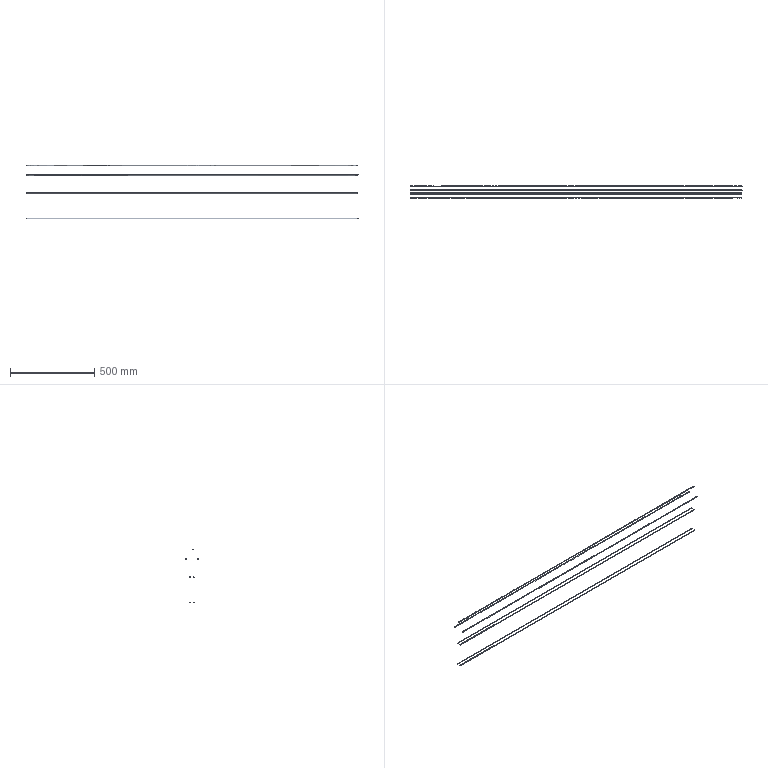Part | SolidWorks | features BaseBody 7 | 7 solids | 28 faces | box 1975 x 72.517 x 321.142 mm | volume 173509 mm3 | spline 14 | plane 14
STEP:
#1=CARTESIAN_POINT('',(28.5,0.007462,-18.003));
#2=VERTEX_POINT('',#1);
#3=CARTESIAN_POINT('',(2000.,0.5236,-17.996));
#4=VERTEX_POINT('',#3);
#5=CARTESIAN_POINT('',(1014.25,0.2655,-18.));
#6=DIRECTION('',(1.,0.0002618,0.000003427));
#7=VECTOR('',#6,1000.);
#8=LINE('',#5,#7);
#9=EDGE_CURVE('',#2,#4,#8,.T.);
#10=ORIENTED_EDGE('',*,*,#9,.F.);
#11=CARTESIAN_POINT('',(28.5,0.007462,-22.003));
#12=VERTEX_POINT('',#11);
#13=CARTESIAN_POINT('',(28.5,0.007462,-22.003));
#14=CARTESIAN_POINT('',(28.5,-3.993,-22.003));
#15=CARTESIAN_POINT('',(28.5,-3.993,-18.003));
#16=CARTESIAN_POINT('',(28.5,0.007462,-18.003));
#17=(BOUNDED_CURVE()B_SPLINE_CURVE(3,(#13,#14,#15,#16),.UNSPECIFIED.,.F.,.F.)B_SPLINE_CURVE_WITH_KNOTS((4,4),(0.,0.006252),.UNSPECIFIED.)CURVE()GEOMETRIC_REPRESENTATION_ITEM()RATIONAL_B_SPLINE_CURVE((1.,0.3333,0.3333,1.))REPRESENTATION_ITEM(''));
#18=EDGE_CURVE('',#12,#2,#17,.T.);
#19=ORIENTED_EDGE('',*,*,#18,.F.);
#20=CARTESIAN_POINT('',(2000.,0.5236,-21.996));
#21=VERTEX_POINT('',#20);
#22=CARTESIAN_POINT('',(1014.25,0.2655,-22.));
#23=DIRECTION('',(-1.,-0.0002618,-0.000003427));
#24=VECTOR('',#23,1000.);
#25=LINE('',#22,#24);
#26=EDGE_CURVE('',#21,#12,#25,.T.);
#27=ORIENTED_EDGE('',*,*,#26,.F.);
#28=CARTESIAN_POINT('',(2000.,0.5236,-17.996));
#29=CARTESIAN_POINT('',(2000.,-3.476,-17.996));
#30=CARTESIAN_POINT('',(2000.,-3.476,-21.996));
#31=CARTESIAN_POINT('',(2000.,0.5236,-21.996));
#32=(BOUNDED_CURVE()B_SPLINE_CURVE(3,(#28,#29,#30,#31),.UNSPECIFIED.,.F.,.F.)B_SPLINE_CURVE_WITH_KNOTS((4,4),(0.,0.006252),.UNSPECIFIED.)CURVE()GEOMETRIC_REPRESENTATION_ITEM()RATIONAL_B_SPLINE_CURVE((1.,0.3333,0.3333,1.))REPRESENTATION_ITEM(''));
#33=EDGE_CURVE('',#4,#21,#32,.T.);
#34=ORIENTED_EDGE('',*,*,#33,.F.);
#35=EDGE_LOOP('',(#10,#19,#27,#34));
#36=FACE_OUTER_BOUND('',#35,.T.);
#37=CARTESIAN_POINT('',(2000.,0.5236,-17.996));
#38=CARTESIAN_POINT('',(28.5,0.007462,-18.003));
#39=CARTESIAN_POINT('',(2000.,-3.476,-17.996));
#40=CARTESIAN_POINT('',(28.5,-3.993,-18.003));
#41=CARTESIAN_POINT('',(2000.,-3.476,-21.996));
#42=CARTESIAN_POINT('',(28.5,-3.993,-22.003));
#43=CARTESIAN_POINT('',(2000.,0.5236,-21.996));
#44=CARTESIAN_POINT('',(28.5,0.007462,-22.003));
#45=(BOUNDED_SURFACE()B_SPLINE_SURFACE(3,1,((#37,#38),(#39,#40),(#41,#42),(#43,#44)),.UNSPECIFIED.,.F.,.F.,.F.)B_SPLINE_SURFACE_WITH_KNOTS((4,4),(2,2),(0.,1.),(0.,1.),.UNSPECIFIED.)GEOMETRIC_REPRESENTATION_ITEM()RATIONAL_B_SPLINE_SURFACE(((1.,1.),(0.3333,0.3333),(0.3333,0.3333),(1.,1.)))REPRESENTATION_ITEM('')SURFACE());
#46=ADVANCED_FACE('',(#36),#45,.F.);
#47=CARTESIAN_POINT('',(2000.,0.5236,-21.996));
#48=CARTESIAN_POINT('',(2000.,4.524,-21.996));
#49=CARTESIAN_POINT('',(2000.,4.524,-17.996));
#50=CARTESIAN_POINT('',(2000.,0.5236,-17.996));
#51=(BOUNDED_CURVE()B_SPLINE_CURVE(3,(#47,#48,#49,#50),.UNSPECIFIED.,.F.,.F.)B_SPLINE_CURVE_WITH_KNOTS((4,4),(0.,0.006252),.UNSPECIFIED.)CURVE()GEOMETRIC_REPRESENTATION_ITEM()RATIONAL_B_SPLINE_CURVE((1.,0.3333,0.3333,1.))REPRESENTATION_ITEM(''));
#52=EDGE_CURVE('',#21,#4,#51,.T.);
#53=ORIENTED_EDGE('',*,*,#52,.T.);
#54=ORIENTED_EDGE('',*,*,#33,.T.);
#55=EDGE_LOOP('',(#53,#54));
#56=FACE_OUTER_BOUND('',#55,.T.);
#57=CARTESIAN_POINT('',(2000.,-1.5,-17.972));
#58=DIRECTION('',(1.,0.,0.));
#59=DIRECTION('',(0.,0.,-1.));
#60=AXIS2_PLACEMENT_3D('',#57,#58,#59);
#61=PLANE('',#60);
#62=ADVANCED_FACE('',(#56),#61,.T.);
#63=ORIENTED_EDGE('',*,*,#52,.F.);
#64=ORIENTED_EDGE('',*,*,#26,.T.);
#65=CARTESIAN_POINT('',(28.5,0.007462,-18.003));
#66=CARTESIAN_POINT('',(28.5,4.007,-18.003));
#67=CARTESIAN_POINT('',(28.5,4.007,-22.003));
#68=CARTESIAN_POINT('',(28.5,0.007462,-22.003));
#69=(BOUNDED_CURVE()B_SPLINE_CURVE(3,(#65,#66,#67,#68),.UNSPECIFIED.,.F.,.F.)B_SPLINE_CURVE_WITH_KNOTS((4,4),(0.,0.006252),.UNSPECIFIED.)CURVE()GEOMETRIC_REPRESENTATION_ITEM()RATIONAL_B_SPLINE_CURVE((1.,0.3333,0.3333,1.))REPRESENTATION_ITEM(''));
#70=EDGE_CURVE('',#2,#12,#69,.T.);
#71=ORIENTED_EDGE('',*,*,#70,.F.);
#72=ORIENTED_EDGE('',*,*,#9,.T.);
#73=EDGE_LOOP('',(#63,#64,#71,#72));
#74=FACE_OUTER_BOUND('',#73,.T.);
#75=CARTESIAN_POINT('',(2000.,0.5236,-21.996));
#76=CARTESIAN_POINT('',(28.5,0.007462,-22.003));
#77=CARTESIAN_POINT('',(2000.,4.524,-21.996));
#78=CARTESIAN_POINT('',(28.5,4.007,-22.003));
#79=CARTESIAN_POINT('',(2000.,4.524,-17.996));
#80=CARTESIAN_POINT('',(28.5,4.007,-18.003));
#81=CARTESIAN_POINT('',(2000.,0.5236,-17.996));
#82=CARTESIAN_POINT('',(28.5,0.007462,-18.003));
#83=(BOUNDED_SURFACE()B_SPLINE_SURFACE(3,1,((#75,#76),(#77,#78),(#79,#80),(#81,#82)),.UNSPECIFIED.,.F.,.F.,.F.)B_SPLINE_SURFACE_WITH_KNOTS((4,4),(2,2),(0.,1.),(0.,1.),.UNSPECIFIED.)GEOMETRIC_REPRESENTATION_ITEM()RATIONAL_B_SPLINE_SURFACE(((1.,1.),(0.3333,0.3333),(0.3333,0.3333),(1.,1.)))REPRESENTATION_ITEM('')SURFACE());
#84=ADVANCED_FACE('',(#74),#83,.F.);
#85=ORIENTED_EDGE('',*,*,#18,.T.);
#86=ORIENTED_EDGE('',*,*,#70,.T.);
#87=EDGE_LOOP('',(#85,#86));
#88=FACE_OUTER_BOUND('',#87,.T.);
#89=CARTESIAN_POINT('',(28.5,-2.017,-22.027));
#90=DIRECTION('',(-1.,0.,0.));
#91=DIRECTION('',(0.,0.,1.));
#92=AXIS2_PLACEMENT_3D('',#89,#90,#91);
#93=PLANE('',#92);
#94=ADVANCED_FACE('',(#88),#93,.T.);
#95=CLOSED_SHELL('',(#46,#62,#84,#94));
#96=MANIFOLD_SOLID_BREP('',#95);
#97=CARTESIAN_POINT('',(28.5,0.007462,-169.026));
#98=VERTEX_POINT('',#97);
#99=CARTESIAN_POINT('',(2000.,0.5236,-169.019));
#100=VERTEX_POINT('',#99);
#101=CARTESIAN_POINT('',(1014.25,0.2655,-169.023));
#102=DIRECTION('',(1.,0.0002618,0.000003427));
#103=VECTOR('',#102,1000.);
#104=LINE('',#101,#103);
#105=EDGE_CURVE('',#98,#100,#104,.T.);
#106=ORIENTED_EDGE('',*,*,#105,.F.);
#107=CARTESIAN_POINT('',(28.5,0.007462,-173.026));
#108=VERTEX_POINT('',#107);
#109=CARTESIAN_POINT('',(28.5,0.007462,-173.026));
#110=CARTESIAN_POINT('',(28.5,-3.993,-173.026));
#111=CARTESIAN_POINT('',(28.5,-3.993,-169.026));
#112=CARTESIAN_POINT('',(28.5,0.007462,-169.026));
#113=(BOUNDED_CURVE()B_SPLINE_CURVE(3,(#109,#110,#111,#112),.UNSPECIFIED.,.F.,.F.)B_SPLINE_CURVE_WITH_KNOTS((4,4),(0.,0.006252),.UNSPECIFIED.)CURVE()GEOMETRIC_REPRESENTATION_ITEM()RATIONAL_B_SPLINE_CURVE((1.,0.3333,0.3333,1.))REPRESENTATION_ITEM(''));
#114=EDGE_CURVE('',#108,#98,#113,.T.);
#115=ORIENTED_EDGE('',*,*,#114,.F.);
#116=CARTESIAN_POINT('',(2000.,0.5236,-173.019));
#117=VERTEX_POINT('',#116);
#118=CARTESIAN_POINT('',(1014.25,0.2655,-173.023));
#119=DIRECTION('',(-1.,-0.0002618,-0.000003427));
#120=VECTOR('',#119,1000.);
#121=LINE('',#118,#120);
#122=EDGE_CURVE('',#117,#108,#121,.T.);
#123=ORIENTED_EDGE('',*,*,#122,.F.);
#124=CARTESIAN_POINT('',(2000.,0.5236,-169.019));
#125=CARTESIAN_POINT('',(2000.,-3.476,-169.019));
#126=CARTESIAN_POINT('',(2000.,-3.476,-173.019));
#127=CARTESIAN_POINT('',(2000.,0.5236,-173.019));
#128=(BOUNDED_CURVE()B_SPLINE_CURVE(3,(#124,#125,#126,#127),.UNSPECIFIED.,.F.,.F.)B_SPLINE_CURVE_WITH_KNOTS((4,4),(0.,0.006252),.UNSPECIFIED.)CURVE()GEOMETRIC_REPRESENTATION_ITEM()RATIONAL_B_SPLINE_CURVE((1.,0.3333,0.3333,1.))REPRESENTATION_ITEM(''));
#129=EDGE_CURVE('',#100,#117,#128,.T.);
#130=ORIENTED_EDGE('',*,*,#129,.F.);
#131=EDGE_LOOP('',(#106,#115,#123,#130));
#132=FACE_OUTER_BOUND('',#131,.T.);
#133=CARTESIAN_POINT('',(2000.,0.5236,-169.019));
#134=CARTESIAN_POINT('',(28.5,0.007462,-169.026));
#135=CARTESIAN_POINT('',(2000.,-3.476,-169.019));
#136=CARTESIAN_POINT('',(28.5,-3.993,-169.026));
#137=CARTESIAN_POINT('',(2000.,-3.476,-173.019));
#138=CARTESIAN_POINT('',(28.5,-3.993,-173.026));
#139=CARTESIAN_POINT('',(2000.,0.5236,-173.019));
#140=CARTESIAN_POINT('',(28.5,0.007462,-173.026));
#141=(BOUNDED_SURFACE()B_SPLINE_SURFACE(3,1,((#133,#134),(#135,#136),(#137,#138),(#139,#140)),.UNSPECIFIED.,.F.,.F.,.T.)B_SPLINE_SURFACE_WITH_KNOTS((4,4),(2,2),(0.,1.),(0.,1.),.UNSPECIFIED.)GEOMETRIC_REPRESENTATION_ITEM()RATIONAL_B_SPLINE_SURFACE(((1.,1.),(0.3333,0.3333),(0.3333,0.3333),(1.,1.)))REPRESENTATION_ITEM('')SURFACE());
#142=ADVANCED_FACE('',(#132),#141,.F.);
#143=CARTESIAN_POINT('',(2000.,0.5236,-173.019));
#144=CARTESIAN_POINT('',(2000.,4.524,-173.019));
#145=CARTESIAN_POINT('',(2000.,4.524,-169.019));
#146=CARTESIAN_POINT('',(2000.,0.5236,-169.019));
#147=(BOUNDED_CURVE()B_SPLINE_CURVE(3,(#143,#144,#145,#146),.UNSPECIFIED.,.F.,.F.)B_SPLINE_CURVE_WITH_KNOTS((4,4),(0.,0.006252),.UNSPECIFIED.)CURVE()GEOMETRIC_REPRESENTATION_ITEM()RATIONAL_B_SPLINE_CURVE((1.,0.3333,0.3333,1.))REPRESENTATION_ITEM(''));
#148=EDGE_CURVE('',#117,#100,#147,.T.);
#149=ORIENTED_EDGE('',*,*,#148,.T.);
#150=ORIENTED_EDGE('',*,*,#129,.T.);
#151=EDGE_LOOP('',(#149,#150));
#152=FACE_OUTER_BOUND('',#151,.T.);
#153=CARTESIAN_POINT('',(2000.,-1.5,-168.995));
#154=DIRECTION('',(1.,0.,0.));
#155=DIRECTION('',(0.,0.,-1.));
#156=AXIS2_PLACEMENT_3D('',#153,#154,#155);
#157=PLANE('',#156);
#158=ADVANCED_FACE('',(#152),#157,.T.);
#159=ORIENTED_EDGE('',*,*,#148,.F.);
#160=ORIENTED_EDGE('',*,*,#122,.T.);
#161=CARTESIAN_POINT('',(28.5,0.007462,-169.026));
#162=CARTESIAN_POINT('',(28.5,4.007,-169.026));
#163=CARTESIAN_POINT('',(28.5,4.007,-173.026));
#164=CARTESIAN_POINT('',(28.5,0.007462,-173.026));
#165=(BOUNDED_CURVE()B_SPLINE_CURVE(3,(#161,#162,#163,#164),.UNSPECIFIED.,.F.,.F.)B_SPLINE_CURVE_WITH_KNOTS((4,4),(0.,0.006252),.UNSPECIFIED.)CURVE()GEOMETRIC_REPRESENTATION_ITEM()RATIONAL_B_SPLINE_CURVE((1.,0.3333,0.3333,1.))REPRESENTATION_ITEM(''));
#166=EDGE_CURVE('',#98,#108,#165,.T.);
#167=ORIENTED_EDGE('',*,*,#166,.F.);
#168=ORIENTED_EDGE('',*,*,#105,.T.);
#169=EDGE_LOOP('',(#159,#160,#167,#168));
#170=FACE_OUTER_BOUND('',#169,.T.);
#171=CARTESIAN_POINT('',(2000.,0.5236,-173.019));
#172=CARTESIAN_POINT('',(28.5,0.007462,-173.026));
#173=CARTESIAN_POINT('',(2000.,4.524,-173.019));
#174=CARTESIAN_POINT('',(28.5,4.007,-173.026));
#175=CARTESIAN_POINT('',(2000.,4.524,-169.019));
#176=CARTESIAN_POINT('',(28.5,4.007,-169.026));
#177=CARTESIAN_POINT('',(2000.,0.5236,-169.019));
#178=CARTESIAN_POINT('',(28.5,0.007462,-169.026));
#179=(BOUNDED_SURFACE()B_SPLINE_SURFACE(3,1,((#171,#172),(#173,#174),(#175,#176),(#177,#178)),.UNSPECIFIED.,.F.,.F.,.F.)B_SPLINE_SURFACE_WITH_KNOTS((4,4),(2,2),(0.,1.),(0.,1.),.UNSPECIFIED.)GEOMETRIC_REPRESENTATION_ITEM()RATIONAL_B_SPLINE_SURFACE(((1.,1.),(0.3333,0.3333),(0.3333,0.3333),(1.,1.)))REPRESENTATION_ITEM('')SURFACE());
#180=ADVANCED_FACE('',(#170),#179,.F.);
#181=ORIENTED_EDGE('',*,*,#114,.T.);
#182=ORIENTED_EDGE('',*,*,#166,.T.);
#183=EDGE_LOOP('',(#181,#182));
#184=FACE_OUTER_BOUND('',#183,.T.);
#185=CARTESIAN_POINT('',(28.5,-2.017,-173.05));
#186=DIRECTION('',(-1.,0.,0.));
#187=DIRECTION('',(0.,0.,1.));
#188=AXIS2_PLACEMENT_3D('',#185,#186,#187);
#189=PLANE('',#188);
#190=ADVANCED_FACE('',(#184),#189,.T.);
#191=CLOSED_SHELL('',(#142,#158,#180,#190));
#192=MANIFOLD_SOLID_BREP('',#191);
#193=CARTESIAN_POINT('',(28.5,22.007,-168.642));
#194=VERTEX_POINT('',#193);
#195=CARTESIAN_POINT('',(2000.,22.524,-168.635));
#196=VERTEX_POINT('',#195);
#197=CARTESIAN_POINT('',(1014.25,22.266,-168.639));
#198=DIRECTION('',(1.,0.0002618,0.000003427));
#199=VECTOR('',#198,1000.);
#200=LINE('',#197,#199);
#201=EDGE_CURVE('',#194,#196,#200,.T.);
#202=ORIENTED_EDGE('',*,*,#201,.F.);
#203=CARTESIAN_POINT('',(28.5,22.007,-172.642));
#204=VERTEX_POINT('',#203);
#205=CARTESIAN_POINT('',(28.5,22.007,-172.642));
#206=CARTESIAN_POINT('',(28.5,18.007,-172.642));
#207=CARTESIAN_POINT('',(28.5,18.007,-168.642));
#208=CARTESIAN_POINT('',(28.5,22.007,-168.642));
#209=(BOUNDED_CURVE()B_SPLINE_CURVE(3,(#205,#206,#207,#208),.UNSPECIFIED.,.F.,.F.)B_SPLINE_CURVE_WITH_KNOTS((4,4),(0.,0.006252),.UNSPECIFIED.)CURVE()GEOMETRIC_REPRESENTATION_ITEM()RATIONAL_B_SPLINE_CURVE((1.,0.3333,0.3333,1.))REPRESENTATION_ITEM(''));
#210=EDGE_CURVE('',#204,#194,#209,.T.);
#211=ORIENTED_EDGE('',*,*,#210,.F.);
#212=CARTESIAN_POINT('',(2000.,22.524,-172.635));
#213=VERTEX_POINT('',#212);
#214=CARTESIAN_POINT('',(1014.25,22.266,-172.639));
#215=DIRECTION('',(-1.,-0.0002618,-0.000003427));
#216=VECTOR('',#215,1000.);
#217=LINE('',#214,#216);
#218=EDGE_CURVE('',#213,#204,#217,.T.);
#219=ORIENTED_EDGE('',*,*,#218,.F.);
#220=CARTESIAN_POINT('',(2000.,22.524,-168.635));
#221=CARTESIAN_POINT('',(2000.,18.524,-168.635));
#222=CARTESIAN_POINT('',(2000.,18.524,-172.635));
#223=CARTESIAN_POINT('',(2000.,22.524,-172.635));
#224=(BOUNDED_CURVE()B_SPLINE_CURVE(3,(#220,#221,#222,#223),.UNSPECIFIED.,.F.,.F.)B_SPLINE_CURVE_WITH_KNOTS((4,4),(0.,0.006252),.UNSPECIFIED.)CURVE()GEOMETRIC_REPRESENTATION_ITEM()RATIONAL_B_SPLINE_CURVE((1.,0.3333,0.3333,1.))REPRESENTATION_ITEM(''));
#225=EDGE_CURVE('',#196,#213,#224,.T.);
#226=ORIENTED_EDGE('',*,*,#225,.F.);
#227=EDGE_LOOP('',(#202,#211,#219,#226));
#228=FACE_OUTER_BOUND('',#227,.T.);
#229=CARTESIAN_POINT('',(2000.,22.524,-168.635));
#230=CARTESIAN_POINT('',(28.5,22.007,-168.642));
#231=CARTESIAN_POINT('',(2000.,18.524,-168.635));
#232=CARTESIAN_POINT('',(28.5,18.007,-168.642));
#233=CARTESIAN_POINT('',(2000.,18.524,-172.635));
#234=CARTESIAN_POINT('',(28.5,18.007,-172.642));
#235=CARTESIAN_POINT('',(2000.,22.524,-172.635));
#236=CARTESIAN_POINT('',(28.5,22.007,-172.642));
#237=(BOUNDED_SURFACE()B_SPLINE_SURFACE(3,1,((#229,#230),(#231,#232),(#233,#234),(#235,#236)),.UNSPECIFIED.,.F.,.F.,.F.)B_SPLINE_SURFACE_WITH_KNOTS((4,4),(2,2),(0.,1.),(0.,1.),.UNSPECIFIED.)GEOMETRIC_REPRESENTATION_ITEM()RATIONAL_B_SPLINE_SURFACE(((1.,1.),(0.3333,0.3333),(0.3333,0.3333),(1.,1.)))REPRESENTATION_ITEM('')SURFACE());
#238=ADVANCED_FACE('',(#228),#237,.F.);
#239=CARTESIAN_POINT('',(2000.,22.524,-172.635));
#240=CARTESIAN_POINT('',(2000.,26.524,-172.635));
#241=CARTESIAN_POINT('',(2000.,26.524,-168.635));
#242=CARTESIAN_POINT('',(2000.,22.524,-168.635));
#243=(BOUNDED_CURVE()B_SPLINE_CURVE(3,(#239,#240,#241,#242),.UNSPECIFIED.,.F.,.F.)B_SPLINE_CURVE_WITH_KNOTS((4,4),(0.,0.006252),.UNSPECIFIED.)CURVE()GEOMETRIC_REPRESENTATION_ITEM()RATIONAL_B_SPLINE_CURVE((1.,0.3333,0.3333,1.))REPRESENTATION_ITEM(''));
#244=EDGE_CURVE('',#213,#196,#243,.T.);
#245=ORIENTED_EDGE('',*,*,#244,.T.);
#246=ORIENTED_EDGE('',*,*,#225,.T.);
#247=EDGE_LOOP('',(#245,#246));
#248=FACE_OUTER_BOUND('',#247,.T.);
#249=CARTESIAN_POINT('',(2000.,20.5,-168.611));
#250=DIRECTION('',(1.,0.,0.));
#251=DIRECTION('',(0.,0.,-1.));
#252=AXIS2_PLACEMENT_3D('',#249,#250,#251);
#253=PLANE('',#252);
#254=ADVANCED_FACE('',(#248),#253,.T.);
#255=ORIENTED_EDGE('',*,*,#244,.F.);
#256=ORIENTED_EDGE('',*,*,#218,.T.);
#257=CARTESIAN_POINT('',(28.5,22.007,-168.642));
#258=CARTESIAN_POINT('',(28.5,26.007,-168.642));
#259=CARTESIAN_POINT('',(28.5,26.007,-172.642));
#260=CARTESIAN_POINT('',(28.5,22.007,-172.642));
#261=(BOUNDED_CURVE()B_SPLINE_CURVE(3,(#257,#258,#259,#260),.UNSPECIFIED.,.F.,.F.)B_SPLINE_CURVE_WITH_KNOTS((4,4),(0.,0.006252),.UNSPECIFIED.)CURVE()GEOMETRIC_REPRESENTATION_ITEM()RATIONAL_B_SPLINE_CURVE((1.,0.3333,0.3333,1.))REPRESENTATION_ITEM(''));
#262=EDGE_CURVE('',#194,#204,#261,.T.);
#263=ORIENTED_EDGE('',*,*,#262,.F.);
#264=ORIENTED_EDGE('',*,*,#201,.T.);
#265=EDGE_LOOP('',(#255,#256,#263,#264));
#266=FACE_OUTER_BOUND('',#265,.T.);
#267=CARTESIAN_POINT('',(2000.,22.524,-172.635));
#268=CARTESIAN_POINT('',(28.5,22.007,-172.642));
#269=CARTESIAN_POINT('',(2000.,26.524,-172.635));
#270=CARTESIAN_POINT('',(28.5,26.007,-172.642));
#271=CARTESIAN_POINT('',(2000.,26.524,-168.635));
#272=CARTESIAN_POINT('',(28.5,26.007,-168.642));
#273=CARTESIAN_POINT('',(2000.,22.524,-168.635));
#274=CARTESIAN_POINT('',(28.5,22.007,-168.642));
#275=(BOUNDED_SURFACE()B_SPLINE_SURFACE(3,1,((#267,#268),(#269,#270),(#271,#272),(#273,#274)),.UNSPECIFIED.,.F.,.F.,.T.)B_SPLINE_SURFACE_WITH_KNOTS((4,4),(2,2),(0.,1.),(0.,1.),.UNSPECIFIED.)GEOMETRIC_REPRESENTATION_ITEM()RATIONAL_B_SPLINE_SURFACE(((1.,1.),(0.3333,0.3333),(0.3333,0.3333),(1.,1.)))REPRESENTATION_ITEM('')SURFACE());
#276=ADVANCED_FACE('',(#266),#275,.F.);
#277=ORIENTED_EDGE('',*,*,#210,.T.);
#278=ORIENTED_EDGE('',*,*,#262,.T.);
#279=EDGE_LOOP('',(#277,#278));
#280=FACE_OUTER_BOUND('',#279,.T.);
#281=CARTESIAN_POINT('',(28.5,19.983,-172.666));
#282=DIRECTION('',(-1.,0.,0.));
#283=DIRECTION('',(0.,0.,1.));
#284=AXIS2_PLACEMENT_3D('',#281,#282,#283);
#285=PLANE('',#284);
#286=ADVANCED_FACE('',(#280),#285,.T.);
#287=CLOSED_SHELL('',(#238,#254,#276,#286));
#288=MANIFOLD_SOLID_BREP('',#287);
#289=CARTESIAN_POINT('',(28.5,22.007,-17.619));
#290=VERTEX_POINT('',#289);
#291=CARTESIAN_POINT('',(2000.,22.524,-17.612));
#292=VERTEX_POINT('',#291);
#293=CARTESIAN_POINT('',(1014.25,22.266,-17.616));
#294=DIRECTION('',(1.,0.0002618,0.000003427));
#295=VECTOR('',#294,1000.);
#296=LINE('',#293,#295);
#297=EDGE_CURVE('',#290,#292,#296,.T.);
#298=ORIENTED_EDGE('',*,*,#297,.F.);
#299=CARTESIAN_POINT('',(28.5,22.007,-21.619));
#300=VERTEX_POINT('',#299);
#301=CARTESIAN_POINT('',(28.5,22.007,-21.619));
#302=CARTESIAN_POINT('',(28.5,18.007,-21.619));
#303=CARTESIAN_POINT('',(28.5,18.007,-17.619));
#304=CARTESIAN_POINT('',(28.5,22.007,-17.619));
#305=(BOUNDED_CURVE()B_SPLINE_CURVE(3,(#301,#302,#303,#304),.UNSPECIFIED.,.F.,.F.)B_SPLINE_CURVE_WITH_KNOTS((4,4),(0.,0.006252),.UNSPECIFIED.)CURVE()GEOMETRIC_REPRESENTATION_ITEM()RATIONAL_B_SPLINE_CURVE((1.,0.3333,0.3333,1.))REPRESENTATION_ITEM(''));
#306=EDGE_CURVE('',#300,#290,#305,.T.);
#307=ORIENTED_EDGE('',*,*,#306,.F.);
#308=CARTESIAN_POINT('',(2000.,22.524,-21.612));
#309=VERTEX_POINT('',#308);
#310=CARTESIAN_POINT('',(1014.25,22.266,-21.616));
#311=DIRECTION('',(-1.,-0.0002618,-0.000003427));
#312=VECTOR('',#311,1000.);
#313=LINE('',#310,#312);
#314=EDGE_CURVE('',#309,#300,#313,.T.);
#315=ORIENTED_EDGE('',*,*,#314,.F.);
#316=CARTESIAN_POINT('',(2000.,22.524,-17.612));
#317=CARTESIAN_POINT('',(2000.,18.524,-17.612));
#318=CARTESIAN_POINT('',(2000.,18.524,-21.612));
#319=CARTESIAN_POINT('',(2000.,22.524,-21.612));
#320=(BOUNDED_CURVE()B_SPLINE_CURVE(3,(#316,#317,#318,#319),.UNSPECIFIED.,.F.,.F.)B_SPLINE_CURVE_WITH_KNOTS((4,4),(0.,0.006252),.UNSPECIFIED.)CURVE()GEOMETRIC_REPRESENTATION_ITEM()RATIONAL_B_SPLINE_CURVE((1.,0.3333,0.3333,1.))REPRESENTATION_ITEM(''));
#321=EDGE_CURVE('',#292,#309,#320,.T.);
#322=ORIENTED_EDGE('',*,*,#321,.F.);
#323=EDGE_LOOP('',(#298,#307,#315,#322));
#324=FACE_OUTER_BOUND('',#323,.T.);
#325=CARTESIAN_POINT('',(2000.,22.524,-17.612));
#326=CARTESIAN_POINT('',(28.5,22.007,-17.619));
#327=CARTESIAN_POINT('',(2000.,18.524,-17.612));
#328=CARTESIAN_POINT('',(28.5,18.007,-17.619));
#329=CARTESIAN_POINT('',(2000.,18.524,-21.612));
#330=CARTESIAN_POINT('',(28.5,18.007,-21.619));
#331=CARTESIAN_POINT('',(2000.,22.524,-21.612));
#332=CARTESIAN_POINT('',(28.5,22.007,-21.619));
#333=(BOUNDED_SURFACE()B_SPLINE_SURFACE(3,1,((#325,#326),(#327,#328),(#329,#330),(#331,#332)),.UNSPECIFIED.,.F.,.F.,.F.)B_SPLINE_SURFACE_WITH_KNOTS((4,4),(2,2),(0.,1.),(0.,1.),.UNSPECIFIED.)GEOMETRIC_REPRESENTATION_ITEM()RATIONAL_B_SPLINE_SURFACE(((1.,1.),(0.3333,0.3333),(0.3333,0.3333),(1.,1.)))REPRESENTATION_ITEM('')SURFACE());
#334=ADVANCED_FACE('',(#324),#333,.F.);
#335=CARTESIAN_POINT('',(2000.,22.524,-21.612));
#336=CARTESIAN_POINT('',(2000.,26.524,-21.612));
#337=CARTESIAN_POINT('',(2000.,26.524,-17.612));
#338=CARTESIAN_POINT('',(2000.,22.524,-17.612));
#339=(BOUNDED_CURVE()B_SPLINE_CURVE(3,(#335,#336,#337,#338),.UNSPECIFIED.,.F.,.F.)B_SPLINE_CURVE_WITH_KNOTS((4,4),(0.,0.006252),.UNSPECIFIED.)CURVE()GEOMETRIC_REPRESENTATION_ITEM()RATIONAL_B_SPLINE_CURVE((1.,0.3333,0.3333,1.))REPRESENTATION_ITEM(''));
#340=EDGE_CURVE('',#309,#292,#339,.T.);
#341=ORIENTED_EDGE('',*,*,#340,.T.);
#342=ORIENTED_EDGE('',*,*,#321,.T.);
#343=EDGE_LOOP('',(#341,#342));
#344=FACE_OUTER_BOUND('',#343,.T.);
#345=CARTESIAN_POINT('',(2000.,20.5,-17.588));
#346=DIRECTION('',(1.,0.,0.));
#347=DIRECTION('',(0.,0.,-1.));
#348=AXIS2_PLACEMENT_3D('',#345,#346,#347);
#349=PLANE('',#348);
#350=ADVANCED_FACE('',(#344),#349,.T.);
#351=ORIENTED_EDGE('',*,*,#340,.F.);
#352=ORIENTED_EDGE('',*,*,#314,.T.);
#353=CARTESIAN_POINT('',(28.5,22.007,-17.619));
#354=CARTESIAN_POINT('',(28.5,26.007,-17.619));
#355=CARTESIAN_POINT('',(28.5,26.007,-21.619));
#356=CARTESIAN_POINT('',(28.5,22.007,-21.619));
#357=(BOUNDED_CURVE()B_SPLINE_CURVE(3,(#353,#354,#355,#356),.UNSPECIFIED.,.F.,.F.)B_SPLINE_CURVE_WITH_KNOTS((4,4),(0.,0.006252),.UNSPECIFIED.)CURVE()GEOMETRIC_REPRESENTATION_ITEM()RATIONAL_B_SPLINE_CURVE((1.,0.3333,0.3333,1.))REPRESENTATION_ITEM(''));
#358=EDGE_CURVE('',#290,#300,#357,.T.);
#359=ORIENTED_EDGE('',*,*,#358,.F.);
#360=ORIENTED_EDGE('',*,*,#297,.T.);
#361=EDGE_LOOP('',(#351,#352,#359,#360));
#362=FACE_OUTER_BOUND('',#361,.T.);
#363=CARTESIAN_POINT('',(2000.,22.524,-21.612));
#364=CARTESIAN_POINT('',(28.5,22.007,-21.619));
#365=CARTESIAN_POINT('',(2000.,26.524,-21.612));
#366=CARTESIAN_POINT('',(28.5,26.007,-21.619));
#367=CARTESIAN_POINT('',(2000.,26.524,-17.612));
#368=CARTESIAN_POINT('',(28.5,26.007,-17.619));
#369=CARTESIAN_POINT('',(2000.,22.524,-17.612));
#370=CARTESIAN_POINT('',(28.5,22.007,-17.619));
#371=(BOUNDED_SURFACE()B_SPLINE_SURFACE(3,1,((#363,#364),(#365,#366),(#367,#368),(#369,#370)),.UNSPECIFIED.,.F.,.F.,.F.)B_SPLINE_SURFACE_WITH_KNOTS((4,4),(2,2),(0.,1.),(0.,1.),.UNSPECIFIED.)GEOMETRIC_REPRESENTATION_ITEM()RATIONAL_B_SPLINE_SURFACE(((1.,1.),(0.3333,0.3333),(0.3333,0.3333),(1.,1.)))REPRESENTATION_ITEM('')SURFACE());
#372=ADVANCED_FACE('',(#362),#371,.F.);
#373=ORIENTED_EDGE('',*,*,#306,.T.);
#374=ORIENTED_EDGE('',*,*,#358,.T.);
#375=EDGE_LOOP('',(#373,#374));
#376=FACE_OUTER_BOUND('',#375,.T.);
#377=CARTESIAN_POINT('',(28.5,19.983,-21.643));
#378=DIRECTION('',(-1.,0.,0.));
#379=DIRECTION('',(0.,0.,1.));
#380=AXIS2_PLACEMENT_3D('',#377,#378,#379);
#381=PLANE('',#380);
#382=ADVANCED_FACE('',(#376),#381,.T.);
#383=CLOSED_SHELL('',(#334,#350,#372,#382));
#384=MANIFOLD_SOLID_BREP('',#383);
#385=CARTESIAN_POINT('',(27.083,-23.993,89.595));
#386=VERTEX_POINT('',#385);
#387=CARTESIAN_POINT('',(2000.,-23.476,89.601));
#388=VERTEX_POINT('',#387);
#389=CARTESIAN_POINT('',(1007.623,-23.736,89.598));
#390=DIRECTION('',(1.,0.0002618,0.000003427));
#391=VECTOR('',#390,1000.);
#392=LINE('',#389,#391);
#393=EDGE_CURVE('',#386,#388,#392,.T.);
#394=ORIENTED_EDGE('',*,*,#393,.F.);
#395=CARTESIAN_POINT('',(27.238,-23.993,85.595));
#396=VERTEX_POINT('',#395);
#397=CARTESIAN_POINT('',(27.238,-23.993,85.595));
#398=CARTESIAN_POINT('',(27.238,-24.125,85.595));
#399=CARTESIAN_POINT('',(27.238,-24.255,85.608));
#400=CARTESIAN_POINT('',(27.236,-24.511,85.658));
#401=CARTESIAN_POINT('',(27.234,-24.638,85.697));
#402=CARTESIAN_POINT('',(27.23,-24.88,85.797));
#403=CARTESIAN_POINT('',(27.228,-24.995,85.859));
#404=CARTESIAN_POINT('',(27.222,-25.212,86.004));
#405=CARTESIAN_POINT('',(27.219,-25.315,86.088));
#406=CARTESIAN_POINT('',(27.208,-25.592,86.365));
#407=CARTESIAN_POINT('',(27.199,-25.741,86.588));
#408=CARTESIAN_POINT('',(27.181,-25.94,87.069));
#409=CARTESIAN_POINT('',(27.171,-25.993,87.332));
#410=CARTESIAN_POINT('',(27.155,-25.993,87.724));
#411=CARTESIAN_POINT('',(27.15,-25.98,87.856));
#412=CARTESIAN_POINT('',(27.14,-25.929,88.112));
#413=CARTESIAN_POINT('',(27.135,-25.891,88.237));
#414=CARTESIAN_POINT('',(27.126,-25.791,88.479));
#415=CARTESIAN_POINT('',(27.121,-25.729,88.596));
#416=CARTESIAN_POINT('',(27.113,-25.584,88.813));
#417=CARTESIAN_POINT('',(27.109,-25.502,88.914));
#418=CARTESIAN_POINT('',(27.102,-25.315,89.101));
#419=CARTESIAN_POINT('',(27.099,-25.214,89.184));
#420=CARTESIAN_POINT('',(27.093,-24.997,89.329));
#421=CARTESIAN_POINT('',(27.09,-24.881,89.392));
#422=CARTESIAN_POINT('',(27.087,-24.638,89.492));
#423=CARTESIAN_POINT('',(27.085,-24.514,89.53));
#424=CARTESIAN_POINT('',(27.083,-24.257,89.581));
#425=CARTESIAN_POINT('',(27.083,-24.125,89.595));
#426=CARTESIAN_POINT('',(27.083,-23.993,89.595));
#427=B_SPLINE_CURVE_WITH_KNOTS('',3,(#397,#398,#399,#400,#401,#402,#403,#404,#405,#406,#407,#408,#409,#410,#411,#412,#413,#414,#415,#416,#417,#418,#419,#420,#421,#422,#423,#424,#425,#426),.UNSPECIFIED.,.F.,.F.,(4,2,2,2,2,2,2,2,2,2,2,2,2,2,4),(0.,0.0003909,0.0007818,0.001173,0.001564,0.002345,0.003127,0.003518,0.003909,0.0043,0.004691,0.005081,0.005472,0.005863,0.006254),.UNSPECIFIED.);
#428=EDGE_CURVE('',#396,#386,#427,.T.);
#429=ORIENTED_EDGE('',*,*,#428,.F.);
#430=CARTESIAN_POINT('',(2000.,-23.476,85.601));
#431=VERTEX_POINT('',#430);
#432=CARTESIAN_POINT('',(1007.623,-23.736,85.598));
#433=DIRECTION('',(-1.,-0.0002618,-0.000003427));
#434=VECTOR('',#433,1000.);
#435=LINE('',#432,#434);
#436=EDGE_CURVE('',#431,#396,#435,.T.);
#437=ORIENTED_EDGE('',*,*,#436,.F.);
#438=CARTESIAN_POINT('',(2000.,-23.476,89.601));
#439=CARTESIAN_POINT('',(2000.,-27.476,89.601));
#440=CARTESIAN_POINT('',(2000.,-27.476,85.601));
#441=CARTESIAN_POINT('',(2000.,-23.476,85.601));
#442=(BOUNDED_CURVE()B_SPLINE_CURVE(3,(#438,#439,#440,#441),.UNSPECIFIED.,.F.,.F.)B_SPLINE_CURVE_WITH_KNOTS((4,4),(0.,0.006252),.UNSPECIFIED.)CURVE()GEOMETRIC_REPRESENTATION_ITEM()RATIONAL_B_SPLINE_CURVE((1.,0.3333,0.3333,1.))REPRESENTATION_ITEM(''));
#443=EDGE_CURVE('',#388,#431,#442,.T.);
#444=ORIENTED_EDGE('',*,*,#443,.F.);
#445=EDGE_LOOP('',(#394,#429,#437,#444));
#446=FACE_OUTER_BOUND('',#445,.T.);
#447=CARTESIAN_POINT('',(2000.,-23.476,89.601));
#448=CARTESIAN_POINT('',(15.245,-23.996,89.595));
#449=CARTESIAN_POINT('',(2000.,-27.476,89.601));
#450=CARTESIAN_POINT('',(15.245,-27.996,89.595));
#451=CARTESIAN_POINT('',(2000.,-27.476,85.601));
#452=CARTESIAN_POINT('',(15.245,-27.996,85.595));
#453=CARTESIAN_POINT('',(2000.,-23.476,85.601));
#454=CARTESIAN_POINT('',(15.245,-23.996,85.595));
#455=(BOUNDED_SURFACE()B_SPLINE_SURFACE(3,1,((#447,#448),(#449,#450),(#451,#452),(#453,#454)),.UNSPECIFIED.,.F.,.F.,.F.)B_SPLINE_SURFACE_WITH_KNOTS((4,4),(2,2),(0.,1.),(0.,1.),.UNSPECIFIED.)GEOMETRIC_REPRESENTATION_ITEM()RATIONAL_B_SPLINE_SURFACE(((1.,1.),(0.3333,0.3333),(0.3333,0.3333),(1.,1.)))REPRESENTATION_ITEM('')SURFACE());
#456=ADVANCED_FACE('',(#446),#455,.F.);
#457=CARTESIAN_POINT('',(2000.,-23.476,85.601));
#458=CARTESIAN_POINT('',(2000.,-19.476,85.601));
#459=CARTESIAN_POINT('',(2000.,-19.476,89.601));
#460=CARTESIAN_POINT('',(2000.,-23.476,89.601));
#461=(BOUNDED_CURVE()B_SPLINE_CURVE(3,(#457,#458,#459,#460),.UNSPECIFIED.,.F.,.F.)B_SPLINE_CURVE_WITH_KNOTS((4,4),(0.,0.006252),.UNSPECIFIED.)CURVE()GEOMETRIC_REPRESENTATION_ITEM()RATIONAL_B_SPLINE_CURVE((1.,0.3333,0.3333,1.))REPRESENTATION_ITEM(''));
#462=EDGE_CURVE('',#431,#388,#461,.T.);
#463=ORIENTED_EDGE('',*,*,#462,.T.);
#464=ORIENTED_EDGE('',*,*,#443,.T.);
#465=EDGE_LOOP('',(#463,#464));
#466=FACE_OUTER_BOUND('',#465,.T.);
#467=CARTESIAN_POINT('',(2000.,-25.5,89.625));
#468=DIRECTION('',(1.,0.,0.));
#469=DIRECTION('',(0.,0.,-1.));
#470=AXIS2_PLACEMENT_3D('',#467,#468,#469);
#471=PLANE('',#470);
#472=ADVANCED_FACE('',(#466),#471,.T.);
#473=ORIENTED_EDGE('',*,*,#462,.F.);
#474=ORIENTED_EDGE('',*,*,#436,.T.);
#475=CARTESIAN_POINT('',(27.083,-23.993,89.595));
#476=CARTESIAN_POINT('',(27.083,-23.861,89.595));
#477=CARTESIAN_POINT('',(27.083,-23.731,89.582));
#478=CARTESIAN_POINT('',(27.085,-23.475,89.531));
#479=CARTESIAN_POINT('',(27.087,-23.348,89.492));
#480=CARTESIAN_POINT('',(27.09,-23.106,89.392));
#481=CARTESIAN_POINT('',(27.093,-22.991,89.33));
#482=CARTESIAN_POINT('',(27.098,-22.774,89.185));
#483=CARTESIAN_POINT('',(27.102,-22.671,89.101));
#484=CARTESIAN_POINT('',(27.113,-22.394,88.824));
#485=CARTESIAN_POINT('',(27.121,-22.245,88.601));
#486=CARTESIAN_POINT('',(27.14,-22.046,88.12));
#487=CARTESIAN_POINT('',(27.15,-21.993,87.857));
#488=CARTESIAN_POINT('',(27.165,-21.993,87.466));
#489=CARTESIAN_POINT('',(27.171,-22.006,87.333));
#490=CARTESIAN_POINT('',(27.18,-22.057,87.077));
#491=CARTESIAN_POINT('',(27.185,-22.094,86.952));
#492=CARTESIAN_POINT('',(27.195,-22.194,86.71));
#493=CARTESIAN_POINT('',(27.199,-22.257,86.593));
#494=CARTESIAN_POINT('',(27.208,-22.402,86.376));
#495=CARTESIAN_POINT('',(27.212,-22.484,86.275));
#496=CARTESIAN_POINT('',(27.219,-22.671,86.088));
#497=CARTESIAN_POINT('',(27.222,-22.772,86.005));
#498=CARTESIAN_POINT('',(27.228,-22.988,85.86));
#499=CARTESIAN_POINT('',(27.23,-23.105,85.798));
#500=CARTESIAN_POINT('',(27.234,-23.348,85.697));
#501=CARTESIAN_POINT('',(27.236,-23.472,85.659));
#502=CARTESIAN_POINT('',(27.238,-23.728,85.608));
#503=CARTESIAN_POINT('',(27.238,-23.861,85.595));
#504=CARTESIAN_POINT('',(27.238,-23.993,85.595));
#505=B_SPLINE_CURVE_WITH_KNOTS('',3,(#475,#476,#477,#478,#479,#480,#481,#482,#483,#484,#485,#486,#487,#488,#489,#490,#491,#492,#493,#494,#495,#496,#497,#498,#499,#500,#501,#502,#503,#504),.UNSPECIFIED.,.F.,.F.,(4,2,2,2,2,2,2,2,2,2,2,2,2,2,4),(0.,0.0003909,0.0007818,0.001173,0.001564,0.002345,0.003127,0.003518,0.003909,0.0043,0.004691,0.005081,0.005472,0.005863,0.006254),.UNSPECIFIED.);
#506=EDGE_CURVE('',#386,#396,#505,.T.);
#507=ORIENTED_EDGE('',*,*,#506,.F.);
#508=ORIENTED_EDGE('',*,*,#393,.T.);
#509=EDGE_LOOP('',(#473,#474,#507,#508));
#510=FACE_OUTER_BOUND('',#509,.T.);
#511=CARTESIAN_POINT('',(2000.,-23.476,85.601));
#512=CARTESIAN_POINT('',(15.245,-23.996,85.595));
#513=CARTESIAN_POINT('',(2000.,-19.476,85.601));
#514=CARTESIAN_POINT('',(15.245,-19.996,85.595));
#515=CARTESIAN_POINT('',(2000.,-19.476,89.601));
#516=CARTESIAN_POINT('',(15.245,-19.996,89.595));
#517=CARTESIAN_POINT('',(2000.,-23.476,89.601));
#518=CARTESIAN_POINT('',(15.245,-23.996,89.595));
#519=(BOUNDED_SURFACE()B_SPLINE_SURFACE(3,1,((#511,#512),(#513,#514),(#515,#516),(#517,#518)),.UNSPECIFIED.,.F.,.F.,.T.)B_SPLINE_SURFACE_WITH_KNOTS((4,4),(2,2),(0.,1.),(0.,1.),.UNSPECIFIED.)GEOMETRIC_REPRESENTATION_ITEM()RATIONAL_B_SPLINE_SURFACE(((1.,1.),(0.3333,0.3333),(0.3333,0.3333),(1.,1.)))REPRESENTATION_ITEM('')SURFACE());
#520=ADVANCED_FACE('',(#510),#519,.F.);
#521=ORIENTED_EDGE('',*,*,#428,.T.);
#522=ORIENTED_EDGE('',*,*,#506,.T.);
#523=EDGE_LOOP('',(#521,#522));
#524=FACE_OUTER_BOUND('',#523,.T.);
#525=CARTESIAN_POINT('',(27.239,-26.018,85.571));
#526=DIRECTION('',(-0.9992,0.,-0.03886));
#527=DIRECTION('',(-0.03886,0.,0.9992));
#528=AXIS2_PLACEMENT_3D('',#525,#526,#527);
#529=PLANE('',#528);
#530=ADVANCED_FACE('',(#524),#529,.T.);
#531=CLOSED_SHELL('',(#456,#472,#520,#530));
#532=MANIFOLD_SOLID_BREP('',#531);
#533=CARTESIAN_POINT('',(27.036,44.007,90.782));
#534=VERTEX_POINT('',#533);
#535=CARTESIAN_POINT('',(2000.,44.524,90.788));
#536=VERTEX_POINT('',#535);
#537=CARTESIAN_POINT('',(1007.599,44.264,90.785));
#538=DIRECTION('',(1.,0.0002618,0.000003427));
#539=VECTOR('',#538,1000.);
#540=LINE('',#537,#539);
#541=EDGE_CURVE('',#534,#536,#540,.T.);
#542=ORIENTED_EDGE('',*,*,#541,.F.);
#543=CARTESIAN_POINT('',(27.192,44.007,86.782));
#544=VERTEX_POINT('',#543);
#545=CARTESIAN_POINT('',(27.192,44.007,86.782));
#546=CARTESIAN_POINT('',(27.192,43.875,86.782));
#547=CARTESIAN_POINT('',(27.191,43.745,86.794));
#548=CARTESIAN_POINT('',(27.189,43.489,86.845));
#549=CARTESIAN_POINT('',(27.188,43.362,86.884));
#550=CARTESIAN_POINT('',(27.184,43.12,86.984));
#551=CARTESIAN_POINT('',(27.182,43.005,87.046));
#552=CARTESIAN_POINT('',(27.176,42.788,87.191));
#553=CARTESIAN_POINT('',(27.173,42.685,87.275));
#554=CARTESIAN_POINT('',(27.162,42.408,87.552));
#555=CARTESIAN_POINT('',(27.153,42.259,87.775));
#556=CARTESIAN_POINT('',(27.135,42.06,88.256));
#557=CARTESIAN_POINT('',(27.124,42.007,88.519));
#558=CARTESIAN_POINT('',(27.109,42.007,88.911));
#559=CARTESIAN_POINT('',(27.104,42.02,89.043));
#560=CARTESIAN_POINT('',(27.094,42.071,89.299));
#561=CARTESIAN_POINT('',(27.089,42.109,89.424));
#562=CARTESIAN_POINT('',(27.08,42.209,89.666));
#563=CARTESIAN_POINT('',(27.075,42.271,89.783));
#564=CARTESIAN_POINT('',(27.067,42.416,90.));
#565=CARTESIAN_POINT('',(27.063,42.498,90.101));
#566=CARTESIAN_POINT('',(27.056,42.685,90.288));
#567=CARTESIAN_POINT('',(27.052,42.786,90.371));
#568=CARTESIAN_POINT('',(27.047,43.003,90.516));
#569=CARTESIAN_POINT('',(27.044,43.119,90.578));
#570=CARTESIAN_POINT('',(27.04,43.362,90.679));
#571=CARTESIAN_POINT('',(27.039,43.486,90.717));
#572=CARTESIAN_POINT('',(27.037,43.743,90.768));
#573=CARTESIAN_POINT('',(27.036,43.875,90.782));
#574=CARTESIAN_POINT('',(27.036,44.007,90.782));
#575=B_SPLINE_CURVE_WITH_KNOTS('',3,(#545,#546,#547,#548,#549,#550,#551,#552,#553,#554,#555,#556,#557,#558,#559,#560,#561,#562,#563,#564,#565,#566,#567,#568,#569,#570,#571,#572,#573,#574),.UNSPECIFIED.,.F.,.F.,(4,2,2,2,2,2,2,2,2,2,2,2,2,2,4),(0.,0.0003909,0.0007818,0.001173,0.001564,0.002345,0.003127,0.003518,0.003909,0.0043,0.004691,0.005081,0.005472,0.005863,0.006254),.UNSPECIFIED.);
#576=EDGE_CURVE('',#544,#534,#575,.T.);
#577=ORIENTED_EDGE('',*,*,#576,.F.);
#578=CARTESIAN_POINT('',(2000.,44.524,86.788));
#579=VERTEX_POINT('',#578);
#580=CARTESIAN_POINT('',(1007.599,44.264,86.785));
#581=DIRECTION('',(-1.,-0.0002618,-0.000003427));
#582=VECTOR('',#581,1000.);
#583=LINE('',#580,#582);
#584=EDGE_CURVE('',#579,#544,#583,.T.);
#585=ORIENTED_EDGE('',*,*,#584,.F.);
#586=CARTESIAN_POINT('',(2000.,44.524,90.788));
#587=CARTESIAN_POINT('',(2000.,40.524,90.788));
#588=CARTESIAN_POINT('',(2000.,40.524,86.788));
#589=CARTESIAN_POINT('',(2000.,44.524,86.788));
#590=(BOUNDED_CURVE()B_SPLINE_CURVE(3,(#586,#587,#588,#589),.UNSPECIFIED.,.F.,.F.)B_SPLINE_CURVE_WITH_KNOTS((4,4),(0.,0.006252),.UNSPECIFIED.)CURVE()GEOMETRIC_REPRESENTATION_ITEM()RATIONAL_B_SPLINE_CURVE((1.,0.3333,0.3333,1.))REPRESENTATION_ITEM(''));
#591=EDGE_CURVE('',#536,#579,#590,.T.);
#592=ORIENTED_EDGE('',*,*,#591,.F.);
#593=EDGE_LOOP('',(#542,#577,#585,#592));
#594=FACE_OUTER_BOUND('',#593,.T.);
#595=CARTESIAN_POINT('',(2000.,44.524,90.788));
#596=CARTESIAN_POINT('',(15.199,44.004,90.781));
#597=CARTESIAN_POINT('',(2000.,40.524,90.788));
#598=CARTESIAN_POINT('',(15.199,40.004,90.781));
#599=CARTESIAN_POINT('',(2000.,40.524,86.788));
#600=CARTESIAN_POINT('',(15.199,40.004,86.781));
#601=CARTESIAN_POINT('',(2000.,44.524,86.788));
#602=CARTESIAN_POINT('',(15.199,44.004,86.781));
#603=(BOUNDED_SURFACE()B_SPLINE_SURFACE(3,1,((#595,#596),(#597,#598),(#599,#600),(#601,#602)),.UNSPECIFIED.,.F.,.F.,.F.)B_SPLINE_SURFACE_WITH_KNOTS((4,4),(2,2),(0.,1.),(0.,1.),.UNSPECIFIED.)GEOMETRIC_REPRESENTATION_ITEM()RATIONAL_B_SPLINE_SURFACE(((1.,1.),(0.3333,0.3333),(0.3333,0.3333),(1.,1.)))REPRESENTATION_ITEM('')SURFACE());
#604=ADVANCED_FACE('',(#594),#603,.F.);
#605=CARTESIAN_POINT('',(2000.,44.524,86.788));
#606=CARTESIAN_POINT('',(2000.,48.524,86.788));
#607=CARTESIAN_POINT('',(2000.,48.524,90.788));
#608=CARTESIAN_POINT('',(2000.,44.524,90.788));
#609=(BOUNDED_CURVE()B_SPLINE_CURVE(3,(#605,#606,#607,#608),.UNSPECIFIED.,.F.,.F.)B_SPLINE_CURVE_WITH_KNOTS((4,4),(0.,0.006252),.UNSPECIFIED.)CURVE()GEOMETRIC_REPRESENTATION_ITEM()RATIONAL_B_SPLINE_CURVE((1.,0.3333,0.3333,1.))REPRESENTATION_ITEM(''));
#610=EDGE_CURVE('',#579,#536,#609,.T.);
#611=ORIENTED_EDGE('',*,*,#610,.T.);
#612=ORIENTED_EDGE('',*,*,#591,.T.);
#613=EDGE_LOOP('',(#611,#612));
#614=FACE_OUTER_BOUND('',#613,.T.);
#615=CARTESIAN_POINT('',(2000.,42.5,90.812));
#616=DIRECTION('',(1.,0.,0.));
#617=DIRECTION('',(0.,0.,-1.));
#618=AXIS2_PLACEMENT_3D('',#615,#616,#617);
#619=PLANE('',#618);
#620=ADVANCED_FACE('',(#614),#619,.T.);
#621=ORIENTED_EDGE('',*,*,#610,.F.);
#622=ORIENTED_EDGE('',*,*,#584,.T.);
#623=CARTESIAN_POINT('',(27.036,44.007,90.782));
#624=CARTESIAN_POINT('',(27.036,44.139,90.782));
#625=CARTESIAN_POINT('',(27.037,44.269,90.769));
#626=CARTESIAN_POINT('',(27.039,44.525,90.718));
#627=CARTESIAN_POINT('',(27.04,44.652,90.679));
#628=CARTESIAN_POINT('',(27.044,44.894,90.579));
#629=CARTESIAN_POINT('',(27.047,45.009,90.517));
#630=CARTESIAN_POINT('',(27.052,45.226,90.372));
#631=CARTESIAN_POINT('',(27.056,45.329,90.288));
#632=CARTESIAN_POINT('',(27.066,45.606,90.011));
#633=CARTESIAN_POINT('',(27.075,45.755,89.788));
#634=CARTESIAN_POINT('',(27.094,45.954,89.307));
#635=CARTESIAN_POINT('',(27.104,46.007,89.044));
#636=CARTESIAN_POINT('',(27.119,46.007,88.652));
#637=CARTESIAN_POINT('',(27.124,45.994,88.52));
#638=CARTESIAN_POINT('',(27.134,45.943,88.264));
#639=CARTESIAN_POINT('',(27.139,45.906,88.139));
#640=CARTESIAN_POINT('',(27.149,45.806,87.897));
#641=CARTESIAN_POINT('',(27.153,45.743,87.78));
#642=CARTESIAN_POINT('',(27.162,45.598,87.563));
#643=CARTESIAN_POINT('',(27.165,45.516,87.462));
#644=CARTESIAN_POINT('',(27.173,45.329,87.275));
#645=CARTESIAN_POINT('',(27.176,45.228,87.192));
#646=CARTESIAN_POINT('',(27.182,45.012,87.047));
#647=CARTESIAN_POINT('',(27.184,44.895,86.985));
#648=CARTESIAN_POINT('',(27.188,44.652,86.884));
#649=CARTESIAN_POINT('',(27.189,44.528,86.846));
#650=CARTESIAN_POINT('',(27.191,44.272,86.795));
#651=CARTESIAN_POINT('',(27.192,44.139,86.782));
#652=CARTESIAN_POINT('',(27.192,44.007,86.782));
#653=B_SPLINE_CURVE_WITH_KNOTS('',3,(#623,#624,#625,#626,#627,#628,#629,#630,#631,#632,#633,#634,#635,#636,#637,#638,#639,#640,#641,#642,#643,#644,#645,#646,#647,#648,#649,#650,#651,#652),.UNSPECIFIED.,.F.,.F.,(4,2,2,2,2,2,2,2,2,2,2,2,2,2,4),(0.,0.0003909,0.0007818,0.001173,0.001564,0.002345,0.003127,0.003518,0.003909,0.0043,0.004691,0.005081,0.005472,0.005863,0.006254),.UNSPECIFIED.);
#654=EDGE_CURVE('',#534,#544,#653,.T.);
#655=ORIENTED_EDGE('',*,*,#654,.F.);
#656=ORIENTED_EDGE('',*,*,#541,.T.);
#657=EDGE_LOOP('',(#621,#622,#655,#656));
#658=FACE_OUTER_BOUND('',#657,.T.);
#659=CARTESIAN_POINT('',(2000.,44.524,86.788));
#660=CARTESIAN_POINT('',(15.199,44.004,86.781));
#661=CARTESIAN_POINT('',(2000.,48.524,86.788));
#662=CARTESIAN_POINT('',(15.199,48.004,86.781));
#663=CARTESIAN_POINT('',(2000.,48.524,90.788));
#664=CARTESIAN_POINT('',(15.199,48.004,90.781));
#665=CARTESIAN_POINT('',(2000.,44.524,90.788));
#666=CARTESIAN_POINT('',(15.199,44.004,90.781));
#667=(BOUNDED_SURFACE()B_SPLINE_SURFACE(3,1,((#659,#660),(#661,#662),(#663,#664),(#665,#666)),.UNSPECIFIED.,.F.,.F.,.T.)B_SPLINE_SURFACE_WITH_KNOTS((4,4),(2,2),(0.,1.),(0.,1.),.UNSPECIFIED.)GEOMETRIC_REPRESENTATION_ITEM()RATIONAL_B_SPLINE_SURFACE(((1.,1.),(0.3333,0.3333),(0.3333,0.3333),(1.,1.)))REPRESENTATION_ITEM('')SURFACE());
#668=ADVANCED_FACE('',(#658),#667,.F.);
#669=ORIENTED_EDGE('',*,*,#576,.T.);
#670=ORIENTED_EDGE('',*,*,#654,.T.);
#671=EDGE_LOOP('',(#669,#670));
#672=FACE_OUTER_BOUND('',#671,.T.);
#673=CARTESIAN_POINT('',(27.193,41.982,86.758));
#674=DIRECTION('',(-0.9992,0.,-0.03886));
#675=DIRECTION('',(-0.03886,0.,0.9992));
#676=AXIS2_PLACEMENT_3D('',#673,#674,#675);
#677=PLANE('',#676);
#678=ADVANCED_FACE('',(#672),#677,.T.);
#679=CLOSED_SHELL('',(#604,#620,#668,#678));
#680=MANIFOLD_SOLID_BREP('',#679);
#681=CARTESIAN_POINT('',(24.807,5.006,148.11));
#682=VERTEX_POINT('',#681);
#683=CARTESIAN_POINT('',(2000.,5.524,148.116));
#684=VERTEX_POINT('',#683);
#685=CARTESIAN_POINT('',(1006.478,5.264,148.113));
#686=DIRECTION('',(1.,0.0002618,0.000003427));
#687=VECTOR('',#686,1000.);
#688=LINE('',#685,#687);
#689=EDGE_CURVE('',#682,#684,#688,.T.);
#690=ORIENTED_EDGE('',*,*,#689,.F.);
#691=CARTESIAN_POINT('',(24.963,5.007,144.11));
#692=VERTEX_POINT('',#691);
#693=CARTESIAN_POINT('',(24.963,5.007,144.11));
#694=CARTESIAN_POINT('',(24.963,4.874,144.11));
#695=CARTESIAN_POINT('',(24.962,4.744,144.123));
#696=CARTESIAN_POINT('',(24.96,4.489,144.173));
#697=CARTESIAN_POINT('',(24.959,4.362,144.212));
#698=CARTESIAN_POINT('',(24.955,4.119,144.312));
#699=CARTESIAN_POINT('',(24.952,4.005,144.374));
#700=CARTESIAN_POINT('',(24.947,3.787,144.519));
#701=CARTESIAN_POINT('',(24.943,3.684,144.603));
#702=CARTESIAN_POINT('',(24.933,3.408,144.88));
#703=CARTESIAN_POINT('',(24.924,3.259,145.103));
#704=CARTESIAN_POINT('',(24.905,3.059,145.584));
#705=CARTESIAN_POINT('',(24.895,3.007,145.848));
#706=CARTESIAN_POINT('',(24.88,3.006,146.239));
#707=CARTESIAN_POINT('',(24.875,3.019,146.371));
#708=CARTESIAN_POINT('',(24.865,3.07,146.627));
#709=CARTESIAN_POINT('',(24.86,3.108,146.752));
#710=CARTESIAN_POINT('',(24.85,3.208,146.994));
#711=CARTESIAN_POINT('',(24.846,3.271,147.111));
#712=CARTESIAN_POINT('',(24.838,3.415,147.328));
#713=CARTESIAN_POINT('',(24.834,3.498,147.429));
#714=CARTESIAN_POINT('',(24.826,3.684,147.616));
#715=CARTESIAN_POINT('',(24.823,3.785,147.699));
#716=CARTESIAN_POINT('',(24.817,4.002,147.844));
#717=CARTESIAN_POINT('',(24.815,4.119,147.907));
#718=CARTESIAN_POINT('',(24.811,4.361,148.007));
#719=CARTESIAN_POINT('',(24.81,4.486,148.045));
#720=CARTESIAN_POINT('',(24.808,4.742,148.096));
#721=CARTESIAN_POINT('',(24.807,4.874,148.11));
#722=CARTESIAN_POINT('',(24.807,5.006,148.11));
#723=B_SPLINE_CURVE_WITH_KNOTS('',3,(#693,#694,#695,#696,#697,#698,#699,#700,#701,#702,#703,#704,#705,#706,#707,#708,#709,#710,#711,#712,#713,#714,#715,#716,#717,#718,#719,#720,#721,#722),.UNSPECIFIED.,.F.,.F.,(4,2,2,2,2,2,2,2,2,2,2,2,2,2,4),(0.,0.0003909,0.0007818,0.001173,0.001564,0.002345,0.003127,0.003518,0.003909,0.0043,0.004691,0.005081,0.005472,0.005863,0.006254),.UNSPECIFIED.);
#724=EDGE_CURVE('',#692,#682,#723,.T.);
#725=ORIENTED_EDGE('',*,*,#724,.F.);
#726=CARTESIAN_POINT('',(2000.,5.524,144.116));
#727=VERTEX_POINT('',#726);
#728=CARTESIAN_POINT('',(1006.478,5.264,144.113));
#729=DIRECTION('',(-1.,-0.0002618,-0.000003427));
#730=VECTOR('',#729,1000.);
#731=LINE('',#728,#730);
#732=EDGE_CURVE('',#727,#692,#731,.T.);
#733=ORIENTED_EDGE('',*,*,#732,.F.);
#734=CARTESIAN_POINT('',(2000.,5.524,148.116));
#735=CARTESIAN_POINT('',(2000.,1.524,148.116));
#736=CARTESIAN_POINT('',(2000.,1.524,144.116));
#737=CARTESIAN_POINT('',(2000.,5.524,144.116));
#738=(BOUNDED_CURVE()B_SPLINE_CURVE(3,(#734,#735,#736,#737),.UNSPECIFIED.,.F.,.F.)B_SPLINE_CURVE_WITH_KNOTS((4,4),(0.,0.006252),.UNSPECIFIED.)CURVE()GEOMETRIC_REPRESENTATION_ITEM()RATIONAL_B_SPLINE_CURVE((1.,0.3333,0.3333,1.))REPRESENTATION_ITEM(''));
#739=EDGE_CURVE('',#684,#727,#738,.T.);
#740=ORIENTED_EDGE('',*,*,#739,.F.);
#741=EDGE_LOOP('',(#690,#725,#733,#740));
#742=FACE_OUTER_BOUND('',#741,.T.);
#743=CARTESIAN_POINT('',(2000.,5.524,148.116));
#744=CARTESIAN_POINT('',(12.956,5.003,148.11));
#745=CARTESIAN_POINT('',(2000.,1.524,148.116));
#746=CARTESIAN_POINT('',(12.956,1.003,148.11));
#747=CARTESIAN_POINT('',(2000.,1.524,144.116));
#748=CARTESIAN_POINT('',(12.956,1.003,144.11));
#749=CARTESIAN_POINT('',(2000.,5.524,144.116));
#750=CARTESIAN_POINT('',(12.956,5.003,144.11));
#751=(BOUNDED_SURFACE()B_SPLINE_SURFACE(3,1,((#743,#744),(#745,#746),(#747,#748),(#749,#750)),.UNSPECIFIED.,.F.,.F.,.F.)B_SPLINE_SURFACE_WITH_KNOTS((4,4),(2,2),(0.,1.),(0.,1.),.UNSPECIFIED.)GEOMETRIC_REPRESENTATION_ITEM()RATIONAL_B_SPLINE_SURFACE(((1.,1.),(0.3333,0.3333),(0.3333,0.3333),(1.,1.)))REPRESENTATION_ITEM('')SURFACE());
#752=ADVANCED_FACE('',(#742),#751,.F.);
#753=CARTESIAN_POINT('',(2000.,5.524,144.116));
#754=CARTESIAN_POINT('',(2000.,9.524,144.116));
#755=CARTESIAN_POINT('',(2000.,9.524,148.116));
#756=CARTESIAN_POINT('',(2000.,5.524,148.116));
#757=(BOUNDED_CURVE()B_SPLINE_CURVE(3,(#753,#754,#755,#756),.UNSPECIFIED.,.F.,.F.)B_SPLINE_CURVE_WITH_KNOTS((4,4),(0.,0.006252),.UNSPECIFIED.)CURVE()GEOMETRIC_REPRESENTATION_ITEM()RATIONAL_B_SPLINE_CURVE((1.,0.3333,0.3333,1.))REPRESENTATION_ITEM(''));
#758=EDGE_CURVE('',#727,#684,#757,.T.);
#759=ORIENTED_EDGE('',*,*,#758,.T.);
#760=ORIENTED_EDGE('',*,*,#739,.T.);
#761=EDGE_LOOP('',(#759,#760));
#762=FACE_OUTER_BOUND('',#761,.T.);
#763=CARTESIAN_POINT('',(2000.,3.5,148.14));
#764=DIRECTION('',(1.,0.,0.));
#765=DIRECTION('',(0.,0.,-1.));
#766=AXIS2_PLACEMENT_3D('',#763,#764,#765);
#767=PLANE('',#766);
#768=ADVANCED_FACE('',(#762),#767,.T.);
#769=ORIENTED_EDGE('',*,*,#758,.F.);
#770=ORIENTED_EDGE('',*,*,#732,.T.);
#771=CARTESIAN_POINT('',(24.807,5.006,148.11));
#772=CARTESIAN_POINT('',(24.807,5.139,148.11));
#773=CARTESIAN_POINT('',(24.808,5.269,148.097));
#774=CARTESIAN_POINT('',(24.81,5.524,148.046));
#775=CARTESIAN_POINT('',(24.811,5.651,148.007));
#776=CARTESIAN_POINT('',(24.815,5.894,147.907));
#777=CARTESIAN_POINT('',(24.817,6.008,147.845));
#778=CARTESIAN_POINT('',(24.823,6.226,147.7));
#779=CARTESIAN_POINT('',(24.826,6.329,147.616));
#780=CARTESIAN_POINT('',(24.837,6.605,147.339));
#781=CARTESIAN_POINT('',(24.846,6.754,147.116));
#782=CARTESIAN_POINT('',(24.864,6.954,146.635));
#783=CARTESIAN_POINT('',(24.875,7.006,146.372));
#784=CARTESIAN_POINT('',(24.89,7.007,145.981));
#785=CARTESIAN_POINT('',(24.895,6.994,145.848));
#786=CARTESIAN_POINT('',(24.905,6.943,145.592));
#787=CARTESIAN_POINT('',(24.91,6.905,145.467));
#788=CARTESIAN_POINT('',(24.919,6.805,145.225));
#789=CARTESIAN_POINT('',(24.924,6.742,145.108));
#790=CARTESIAN_POINT('',(24.932,6.598,144.891));
#791=CARTESIAN_POINT('',(24.936,6.515,144.79));
#792=CARTESIAN_POINT('',(24.943,6.329,144.603));
#793=CARTESIAN_POINT('',(24.947,6.228,144.52));
#794=CARTESIAN_POINT('',(24.952,6.011,144.375));
#795=CARTESIAN_POINT('',(24.955,5.894,144.313));
#796=CARTESIAN_POINT('',(24.959,5.652,144.212));
#797=CARTESIAN_POINT('',(24.96,5.527,144.174));
#798=CARTESIAN_POINT('',(24.962,5.271,144.123));
#799=CARTESIAN_POINT('',(24.963,5.139,144.11));
#800=CARTESIAN_POINT('',(24.963,5.007,144.11));
#801=B_SPLINE_CURVE_WITH_KNOTS('',3,(#771,#772,#773,#774,#775,#776,#777,#778,#779,#780,#781,#782,#783,#784,#785,#786,#787,#788,#789,#790,#791,#792,#793,#794,#795,#796,#797,#798,#799,#800),.UNSPECIFIED.,.F.,.F.,(4,2,2,2,2,2,2,2,2,2,2,2,2,2,4),(0.,0.0003909,0.0007818,0.001173,0.001564,0.002345,0.003127,0.003518,0.003909,0.0043,0.004691,0.005081,0.005472,0.005863,0.006254),.UNSPECIFIED.);
#802=EDGE_CURVE('',#682,#692,#801,.T.);
#803=ORIENTED_EDGE('',*,*,#802,.F.);
#804=ORIENTED_EDGE('',*,*,#689,.T.);
#805=EDGE_LOOP('',(#769,#770,#803,#804));
#806=FACE_OUTER_BOUND('',#805,.T.);
#807=CARTESIAN_POINT('',(2000.,5.524,144.116));
#808=CARTESIAN_POINT('',(12.956,5.003,144.11));
#809=CARTESIAN_POINT('',(2000.,9.524,144.116));
#810=CARTESIAN_POINT('',(12.956,9.003,144.11));
#811=CARTESIAN_POINT('',(2000.,9.524,148.116));
#812=CARTESIAN_POINT('',(12.956,9.003,148.11));
#813=CARTESIAN_POINT('',(2000.,5.524,148.116));
#814=CARTESIAN_POINT('',(12.956,5.003,148.11));
#815=(BOUNDED_SURFACE()B_SPLINE_SURFACE(3,1,((#807,#808),(#809,#810),(#811,#812),(#813,#814)),.UNSPECIFIED.,.F.,.F.,.T.)B_SPLINE_SURFACE_WITH_KNOTS((4,4),(2,2),(0.,1.),(0.,1.),.UNSPECIFIED.)GEOMETRIC_REPRESENTATION_ITEM()RATIONAL_B_SPLINE_SURFACE(((1.,1.),(0.3333,0.3333),(0.3333,0.3333),(1.,1.)))REPRESENTATION_ITEM('')SURFACE());
#816=ADVANCED_FACE('',(#806),#815,.F.);
#817=ORIENTED_EDGE('',*,*,#724,.T.);
#818=ORIENTED_EDGE('',*,*,#802,.T.);
#819=EDGE_LOOP('',(#817,#818));
#820=FACE_OUTER_BOUND('',#819,.T.);
#821=CARTESIAN_POINT('',(24.964,2.982,144.086));
#822=DIRECTION('',(-0.9992,0.,-0.03886));
#823=DIRECTION('',(-0.03886,0.,0.9992));
#824=AXIS2_PLACEMENT_3D('',#821,#822,#823);
#825=PLANE('',#824);
#826=ADVANCED_FACE('',(#820),#825,.T.);
#827=CLOSED_SHELL('',(#752,#768,#816,#826));
#828=MANIFOLD_SOLID_BREP('',#827);
#829=CARTESIAN_POINT('',(0.,0.,0.));
#830=DIRECTION('',(0.,0.,1.));
#831=DIRECTION('',(1.,0.,0.));
#832=AXIS2_PLACEMENT_3D('',#829,#830,#831);
#833=(LENGTH_UNIT()NAMED_UNIT(*)SI_UNIT(.MILLI.,.METRE.));
#834=UNCERTAINTY_MEASURE_WITH_UNIT(LENGTH_MEASURE(0.00001),#833,'','');
#835=(NAMED_UNIT(*)PLANE_ANGLE_UNIT()SI_UNIT($,.RADIAN.));
#836=(NAMED_UNIT(*)SI_UNIT($,.STERADIAN.)SOLID_ANGLE_UNIT());
#837=(GEOMETRIC_REPRESENTATION_CONTEXT(3)GLOBAL_UNCERTAINTY_ASSIGNED_CONTEXT((#834))GLOBAL_UNIT_ASSIGNED_CONTEXT((#833,#835,#836))REPRESENTATION_CONTEXT('',''));
#838=ADVANCED_BREP_SHAPE_REPRESENTATION('',(#96,#192,#288,#384,#532,#680,#828,#832),#837);